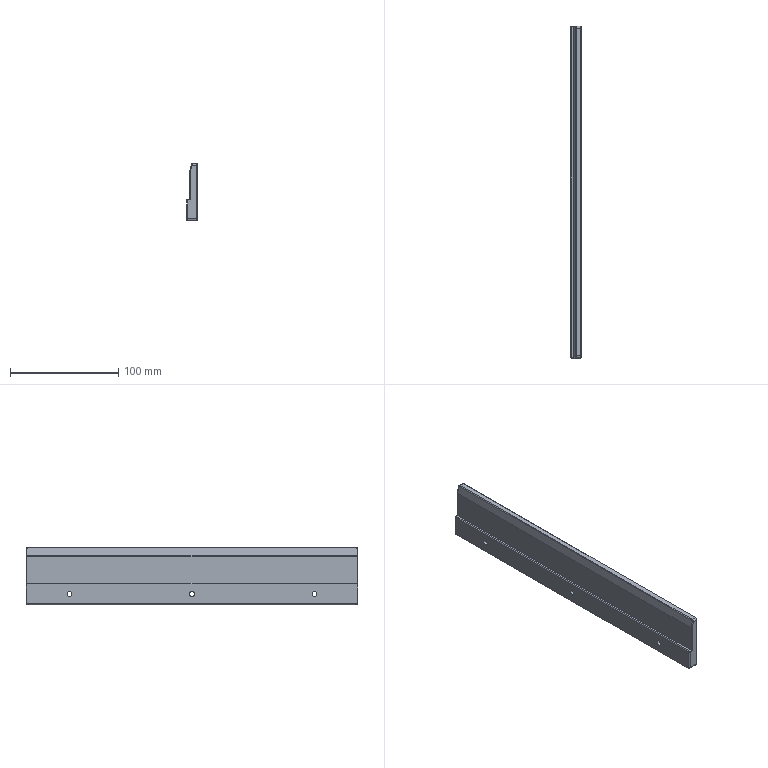CAM job | NX | 3-axis milling | part box 10 x 306 x 53 mm | stock box 12 x 311 x 58 mm
Tools:
number,name,description,diameter,corner_radius,flute_length,length,flutes
9,D10,平底铣刀-粗,10.0,0.0,35.0,75.0,2
10,D10-J,平底铣刀-精,10.0,0.0,35.0,75.0,2
17,D6R0.5,圆鼻刀-粗,6.0,0.5,50.0,75.0,2
1,D80R0.8飞刀,圆鼻刀-粗,80.0,0.8,50.0,75.0,2
2,D6倒角刀,倒角刀,6.0,0.0,3.0,25.0,2
Operations:
program,operation,operation_type,tool,method,geometry_group,spindle_rpm,surface_speed,feed_per_tooth,feed_cut,feed_plunge,cut_length_mm,path_length_mm,cut_time_min,machine_time_min
B,面铣自动飞面开粗_COPY,FaceMilling,D10,分层开粗-切深K-步距G,W-B,8000.0,251.327,0.25,4000.0,100.0,5992.661,6165.616,1.498,1.516
B,面铣自动飞面精光_COPY,FaceMilling,D10-J,侧刃精光-切深K-步距G,W-B,7000.0,219.911,0.0714,1000.0,100.0,666.667,762.667,0.6667,0.6763
B,等高精光往复爬面_COPY_COPY_1,ZLevelMilling,D6R0.5,等高爬面-切深K-步距G,W-B,7000.0,131.947,0.2857,4000.0,100.0,1828.516,2187.438,0.4571,0.493
B,等高精光往复爬面_COPY_COPY_1_COPY,ZLevelMilling,D6R0.5,等高爬面-切深K-步距G,W-B,7000.0,131.947,0.2857,4000.0,100.0,6090.286,6120.149,1.523,1.526
B,底壁铣倒角_COPY_1,VolumeBased25DMillingOperation,D6倒角刀,爬面_倒角-切深0-步距G,W-B,6500.0,122.519,0.1154,1500.0,100.0,311.482,410.882,0.2077,0.2176
A,顶面,FaceMilling,D80R0.8飞刀,侧刃精光-切深K-步距G,W-A,4000.0,1005.31,0.125,1000.0,100.0,400.0,436.0,0.4,0.4036
A,外形粗_2,VolumeBased25DMillingOperation,D10,METHOD,W-A,5000.0,157.08,0.5,5000.0,80.0,45735.743,45827.543,9.147,9.156
A,等高往复层切开粗-中_COPY,ZLevelMilling,D10,分层开粗-切深K-步距G,W-A,5000.0,157.08,0.4,4000.0,100.0,18313.066,19282.325,4.578,4.675
A,底壁铣倒角_COPY,VolumeBased25DMillingOperation,D6倒角刀,爬面_倒角-切深0-步距G,W-A,6500.0,122.519,0.1154,1500.0,100.0,323.254,362.654,0.2155,0.2194
A,等高精光往复爬面_COPY,ZLevelMilling,D6R0.5,等高爬面-切深K-步距G,W-A,7000.0,131.947,0.2857,4000.0,100.0,1418.998,1766.119,0.3547,0.3895
A,等高精光往复爬面_COPY_COPY,ZLevelMilling,D6R0.5,等高爬面-切深K-步距G,W-A,7000.0,131.947,0.2857,4000.0,100.0,32536.24,32565.443,8.134,8.137
A,等高精光-中_COPY,ZLevelMilling,D10-J,侧刃精光-切深K-步距G,W-A,5000.0,157.08,0.1,1000.0,100.0,4322.042,4621.956,4.322,4.352
A,等高精光往复爬面_COPY_COPY_COPY,ZLevelMilling,D10-J,等高爬面-切深K-步距G,W-A,5000.0,157.08,0.4,4000.0,100.0,22665.87,22753.128,5.667,5.675